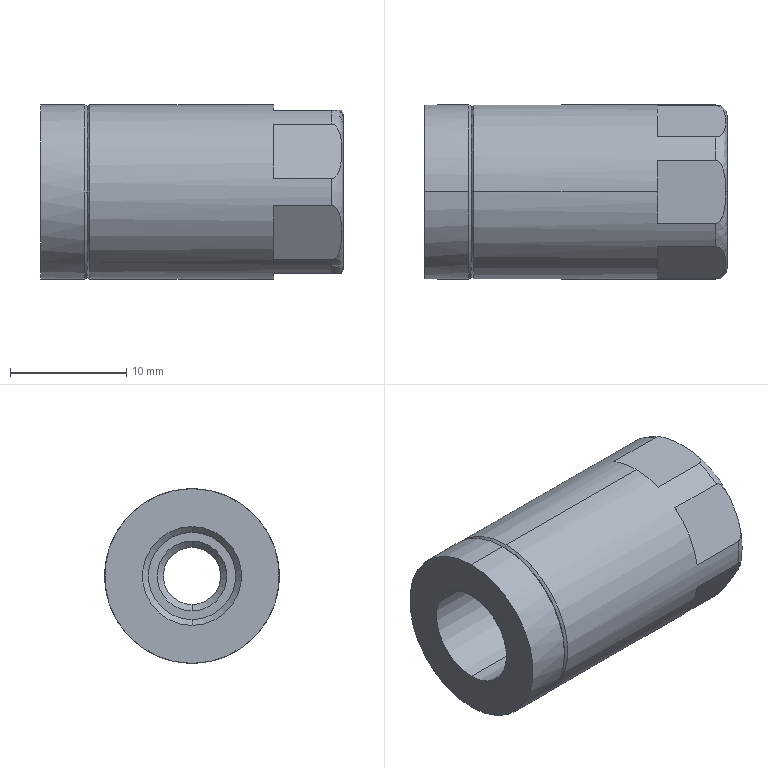Part | STEP file | _ACQJ-16x10_stoper | 1 solid | 35 faces | box 26 x 15 x 15 mm | volume 3348 mm3 | plane 15 | cone 10 | cylinder 8 | spline 2 | commonest cylinder face diameters 15 x4 4.917 x2 8.5 x2
STEP:
#1=CARTESIAN_POINT('',(26.,0.,-6.5));
#2=VERTEX_POINT('',#1);
#3=CARTESIAN_POINT('',(26.,0.,6.5));
#4=VERTEX_POINT('',#3);
#5=CARTESIAN_POINT('',(26.,0.,-6.5));
#6=CARTESIAN_POINT('',(26.,-13.,-6.5));
#7=CARTESIAN_POINT('',(26.,-13.,6.5));
#8=CARTESIAN_POINT('',(26.,0.,6.5));
#9=(BOUNDED_CURVE()B_SPLINE_CURVE(3,(#5,#6,#7,#8),.UNSPECIFIED.,.F.,.T.)B_SPLINE_CURVE_WITH_KNOTS((4,4),(0.,0.5),.UNSPECIFIED.)CURVE()GEOMETRIC_REPRESENTATION_ITEM()RATIONAL_B_SPLINE_CURVE((1.,0.3333,0.3333,1.))REPRESENTATION_ITEM(''));
#10=EDGE_CURVE('',#2,#4,#9,.T.);
#11=ORIENTED_EDGE('',*,*,#10,.T.);
#12=CARTESIAN_POINT('',(25.866,0.,7.));
#13=VERTEX_POINT('',#12);
#14=CARTESIAN_POINT('',(25.,0.,6.5));
#15=DIRECTION('',(0.,-1.,0.));
#16=DIRECTION('',(0.,0.,1.));
#17=AXIS2_PLACEMENT_3D('',#14,#15,#16);
#18=CIRCLE('',#17,1.);
#19=EDGE_CURVE('',#4,#13,#18,.T.);
#20=ORIENTED_EDGE('',*,*,#19,.T.);
#21=CARTESIAN_POINT('',(25.,-2.693,7.));
#22=VERTEX_POINT('',#21);
#23=CARTESIAN_POINT('',(25.866,0.,7.));
#24=CARTESIAN_POINT('',(25.866,-0.2506,7.));
#25=CARTESIAN_POINT('',(25.859,-0.5008,7.));
#26=CARTESIAN_POINT('',(25.825,-0.9999,7.));
#27=CARTESIAN_POINT('',(25.798,-1.249,7.));
#28=CARTESIAN_POINT('',(25.708,-1.744,7.));
#29=CARTESIAN_POINT('',(25.645,-1.991,7.));
#30=CARTESIAN_POINT('',(25.485,-2.33,7.));
#31=CARTESIAN_POINT('',(25.42,-2.44,7.));
#32=CARTESIAN_POINT('',(25.287,-2.576,7.));
#33=CARTESIAN_POINT('',(25.238,-2.616,7.));
#34=CARTESIAN_POINT('',(25.126,-2.675,7.));
#35=CARTESIAN_POINT('',(25.064,-2.693,7.));
#36=CARTESIAN_POINT('',(25.,-2.693,7.));
#37=B_SPLINE_CURVE_WITH_KNOTS('',3,(#23,#24,#25,#26,#27,#28,#29,#30,#31,#32,#33,#34,#35,#36),.UNSPECIFIED.,.F.,.F.,(4,2,2,2,2,2,4),(0.003036,0.003796,0.004556,0.005316,0.005696,0.005886,0.006076),.UNSPECIFIED.);
#38=EDGE_CURVE('',#13,#22,#37,.T.);
#39=ORIENTED_EDGE('',*,*,#38,.T.);
#40=CARTESIAN_POINT('',(25.,-4.716,5.832));
#41=VERTEX_POINT('',#40);
#42=CARTESIAN_POINT('',(25.,0.,0.));
#43=DIRECTION('',(-1.,0.,0.));
#44=DIRECTION('',(0.,0.,1.));
#45=AXIS2_PLACEMENT_3D('',#42,#43,#44);
#46=CIRCLE('',#45,7.5);
#47=EDGE_CURVE('',#41,#22,#46,.T.);
#48=ORIENTED_EDGE('',*,*,#47,.F.);
#49=CARTESIAN_POINT('',(25.,-7.408,1.168));
#50=VERTEX_POINT('',#49);
#51=CARTESIAN_POINT('',(25.,-4.716,5.832));
#52=CARTESIAN_POINT('',(25.064,-4.716,5.832));
#53=CARTESIAN_POINT('',(25.127,-4.725,5.816));
#54=CARTESIAN_POINT('',(25.239,-4.754,5.765));
#55=CARTESIAN_POINT('',(25.289,-4.775,5.73));
#56=CARTESIAN_POINT('',(25.421,-4.843,5.611));
#57=CARTESIAN_POINT('',(25.487,-4.899,5.515));
#58=CARTESIAN_POINT('',(25.594,-5.012,5.318));
#59=CARTESIAN_POINT('',(25.635,-5.072,5.214));
#60=CARTESIAN_POINT('',(25.704,-5.194,5.004));
#61=CARTESIAN_POINT('',(25.731,-5.255,4.898));
#62=CARTESIAN_POINT('',(25.798,-5.439,4.579));
#63=CARTESIAN_POINT('',(25.825,-5.563,4.364));
#64=CARTESIAN_POINT('',(25.859,-5.812,3.933));
#65=CARTESIAN_POINT('',(25.866,-5.938,3.715));
#66=CARTESIAN_POINT('',(25.866,-6.188,3.282));
#67=CARTESIAN_POINT('',(25.859,-6.313,3.065));
#68=CARTESIAN_POINT('',(25.824,-6.563,2.633));
#69=CARTESIAN_POINT('',(25.798,-6.687,2.417));
#70=CARTESIAN_POINT('',(25.707,-6.935,1.989));
#71=CARTESIAN_POINT('',(25.645,-7.058,1.776));
#72=CARTESIAN_POINT('',(25.485,-7.227,1.482));
#73=CARTESIAN_POINT('',(25.419,-7.282,1.387));
#74=CARTESIAN_POINT('',(25.287,-7.35,1.269));
#75=CARTESIAN_POINT('',(25.238,-7.37,1.234));
#76=CARTESIAN_POINT('',(25.126,-7.4,1.183));
#77=CARTESIAN_POINT('',(25.064,-7.408,1.168));
#78=CARTESIAN_POINT('',(25.,-7.408,1.168));
#79=B_SPLINE_CURVE_WITH_KNOTS('',3,(#51,#52,#53,#54,#55,#56,#57,#58,#59,#60,#61,#62,#63,#64,#65,#66,#67,#68,#69,#70,#71,#72,#73,#74,#75,#76,#77,#78),.UNSPECIFIED.,.F.,.F.,(4,2,2,2,2,2,2,2,2,2,2,2,2,4),(0.,0.0001899,0.0003798,0.0007595,0.001139,0.001519,0.002279,0.003038,0.003798,0.004557,0.005317,0.005697,0.005887,0.006076),.UNSPECIFIED.);
#80=EDGE_CURVE('',#41,#50,#79,.T.);
#81=ORIENTED_EDGE('',*,*,#80,.T.);
#82=CARTESIAN_POINT('',(25.,-7.408,-1.168));
#83=VERTEX_POINT('',#82);
#84=CARTESIAN_POINT('',(25.,0.,0.));
#85=DIRECTION('',(-1.,0.,0.));
#86=DIRECTION('',(0.,0.,1.));
#87=AXIS2_PLACEMENT_3D('',#84,#85,#86);
#88=CIRCLE('',#87,7.5);
#89=EDGE_CURVE('',#83,#50,#88,.T.);
#90=ORIENTED_EDGE('',*,*,#89,.F.);
#91=CARTESIAN_POINT('',(25.,-4.716,-5.832));
#92=VERTEX_POINT('',#91);
#93=CARTESIAN_POINT('',(25.,-7.408,-1.168));
#94=CARTESIAN_POINT('',(25.064,-7.408,-1.168));
#95=CARTESIAN_POINT('',(25.127,-7.4,-1.184));
#96=CARTESIAN_POINT('',(25.239,-7.37,-1.235));
#97=CARTESIAN_POINT('',(25.289,-7.35,-1.27));
#98=CARTESIAN_POINT('',(25.421,-7.281,-1.389));
#99=CARTESIAN_POINT('',(25.487,-7.226,-1.485));
#100=CARTESIAN_POINT('',(25.594,-7.112,-1.682));
#101=CARTESIAN_POINT('',(25.635,-7.052,-1.786));
#102=CARTESIAN_POINT('',(25.704,-6.931,-1.996));
#103=CARTESIAN_POINT('',(25.731,-6.87,-2.102));
#104=CARTESIAN_POINT('',(25.798,-6.685,-2.421));
#105=CARTESIAN_POINT('',(25.825,-6.561,-2.636));
#106=CARTESIAN_POINT('',(25.859,-6.312,-3.067));
#107=CARTESIAN_POINT('',(25.866,-6.187,-3.285));
#108=CARTESIAN_POINT('',(25.866,-5.936,-3.718));
#109=CARTESIAN_POINT('',(25.859,-5.811,-3.935));
#110=CARTESIAN_POINT('',(25.824,-5.562,-4.367));
#111=CARTESIAN_POINT('',(25.798,-5.437,-4.583));
#112=CARTESIAN_POINT('',(25.707,-5.19,-5.011));
#113=CARTESIAN_POINT('',(25.645,-5.067,-5.224));
#114=CARTESIAN_POINT('',(25.485,-4.897,-5.518));
#115=CARTESIAN_POINT('',(25.419,-4.842,-5.613));
#116=CARTESIAN_POINT('',(25.287,-4.774,-5.731));
#117=CARTESIAN_POINT('',(25.238,-4.754,-5.766));
#118=CARTESIAN_POINT('',(25.126,-4.725,-5.817));
#119=CARTESIAN_POINT('',(25.064,-4.716,-5.832));
#120=CARTESIAN_POINT('',(25.,-4.716,-5.832));
#121=B_SPLINE_CURVE_WITH_KNOTS('',3,(#93,#94,#95,#96,#97,#98,#99,#100,#101,#102,#103,#104,#105,#106,#107,#108,#109,#110,#111,#112,#113,#114,#115,#116,#117,#118,#119,#120),.UNSPECIFIED.,.F.,.F.,(4,2,2,2,2,2,2,2,2,2,2,2,2,4),(0.,0.0001899,0.0003798,0.0007595,0.001139,0.001519,0.002279,0.003038,0.003798,0.004557,0.005317,0.005697,0.005887,0.006076),.UNSPECIFIED.);
#122=EDGE_CURVE('',#83,#92,#121,.T.);
#123=ORIENTED_EDGE('',*,*,#122,.T.);
#124=CARTESIAN_POINT('',(25.,-2.693,-7.));
#125=VERTEX_POINT('',#124);
#126=CARTESIAN_POINT('',(25.,0.,0.));
#127=DIRECTION('',(-1.,0.,0.));
#128=DIRECTION('',(0.,0.,1.));
#129=AXIS2_PLACEMENT_3D('',#126,#127,#128);
#130=CIRCLE('',#129,7.5);
#131=EDGE_CURVE('',#125,#92,#130,.T.);
#132=ORIENTED_EDGE('',*,*,#131,.F.);
#133=CARTESIAN_POINT('',(25.866,0.,-7.));
#134=VERTEX_POINT('',#133);
#135=CARTESIAN_POINT('',(25.,-2.693,-7.));
#136=CARTESIAN_POINT('',(25.064,-2.693,-7.));
#137=CARTESIAN_POINT('',(25.127,-2.675,-7.));
#138=CARTESIAN_POINT('',(25.239,-2.616,-7.));
#139=CARTESIAN_POINT('',(25.289,-2.575,-7.));
#140=CARTESIAN_POINT('',(25.421,-2.438,-7.));
#141=CARTESIAN_POINT('',(25.486,-2.327,-7.));
#142=CARTESIAN_POINT('',(25.593,-2.1,-7.));
#143=CARTESIAN_POINT('',(25.635,-1.98,-7.));
#144=CARTESIAN_POINT('',(25.704,-1.738,-7.));
#145=CARTESIAN_POINT('',(25.731,-1.616,-7.));
#146=CARTESIAN_POINT('',(25.798,-1.247,-7.));
#147=CARTESIAN_POINT('',(25.825,-0.9993,-7.));
#148=CARTESIAN_POINT('',(25.859,-0.5011,-7.));
#149=CARTESIAN_POINT('',(25.866,-0.2503,-7.));
#150=CARTESIAN_POINT('',(25.866,0.,-7.));
#151=B_SPLINE_CURVE_WITH_KNOTS('',3,(#135,#136,#137,#138,#139,#140,#141,#142,#143,#144,#145,#146,#147,#148,#149,#150),.UNSPECIFIED.,.F.,.F.,(4,2,2,2,2,2,2,4),(0.,0.0001898,0.0003795,0.0007591,0.001139,0.001518,0.002277,0.003036),.UNSPECIFIED.);
#152=EDGE_CURVE('',#125,#134,#151,.T.);
#153=ORIENTED_EDGE('',*,*,#152,.T.);
#154=CARTESIAN_POINT('',(25.,0.,-6.5));
#155=DIRECTION('',(0.,1.,0.));
#156=DIRECTION('',(0.,0.,-1.));
#157=AXIS2_PLACEMENT_3D('',#154,#155,#156);
#158=CIRCLE('',#157,1.);
#159=EDGE_CURVE('',#2,#134,#158,.T.);
#160=ORIENTED_EDGE('',*,*,#159,.F.);
#161=EDGE_LOOP('',(#11,#20,#39,#48,#81,#90,#123,#132,#153,#160));
#162=FACE_OUTER_BOUND('',#161,.T.);
#163=CARTESIAN_POINT('',(26.,0.,6.5));
#164=CARTESIAN_POINT('',(26.,-13.,6.5));
#165=CARTESIAN_POINT('',(26.,-13.,-6.5));
#166=CARTESIAN_POINT('',(26.,0.,-6.5));
#167=CARTESIAN_POINT('',(26.,0.,7.086));
#168=CARTESIAN_POINT('',(26.,-14.172,7.086));
#169=CARTESIAN_POINT('',(26.,-14.172,-7.086));
#170=CARTESIAN_POINT('',(26.,0.,-7.086));
#171=CARTESIAN_POINT('',(25.586,0.,7.5));
#172=CARTESIAN_POINT('',(25.586,-15.,7.5));
#173=CARTESIAN_POINT('',(25.586,-15.,-7.5));
#174=CARTESIAN_POINT('',(25.586,0.,-7.5));
#175=CARTESIAN_POINT('',(25.,0.,7.5));
#176=CARTESIAN_POINT('',(25.,-15.,7.5));
#177=CARTESIAN_POINT('',(25.,-15.,-7.5));
#178=CARTESIAN_POINT('',(25.,0.,-7.5));
#179=(BOUNDED_SURFACE()B_SPLINE_SURFACE(3,3,((#163,#164,#165,#166),(#167,#168,#169,#170),(#171,#172,#173,#174),(#175,#176,#177,#178)),.UNSPECIFIED.,.F.,.F.,.F.)B_SPLINE_SURFACE_WITH_KNOTS((4,4),(4,4),(0.,1.),(0.,1.),.UNSPECIFIED.)GEOMETRIC_REPRESENTATION_ITEM()RATIONAL_B_SPLINE_SURFACE(((1.,0.3333,0.3333,1.),(0.8047,0.2682,0.2682,0.8047),(0.8047,0.2682,0.2682,0.8047),(1.,0.3333,0.3333,1.)))REPRESENTATION_ITEM('')SURFACE());
#180=ADVANCED_FACE('',(#162),#179,.T.);
#181=CARTESIAN_POINT('',(20.,2.693,-7.));
#182=VERTEX_POINT('',#181);
#183=CARTESIAN_POINT('',(20.,0.,-7.5));
#184=VERTEX_POINT('',#183);
#185=CARTESIAN_POINT('',(20.,0.,0.));
#186=DIRECTION('',(-1.,0.,0.));
#187=DIRECTION('',(0.,0.,1.));
#188=AXIS2_PLACEMENT_3D('',#185,#186,#187);
#189=CIRCLE('',#188,7.5);
#190=EDGE_CURVE('',#182,#184,#189,.T.);
#191=ORIENTED_EDGE('',*,*,#190,.T.);
#192=CARTESIAN_POINT('',(4.2,0.,-7.5));
#193=VERTEX_POINT('',#192);
#194=CARTESIAN_POINT('',(26.,0.,-7.5));
#195=DIRECTION('',(-1.,0.,0.));
#196=VECTOR('',#195,1000.);
#197=LINE('',#194,#196);
#198=EDGE_CURVE('',#184,#193,#197,.T.);
#199=ORIENTED_EDGE('',*,*,#198,.T.);
#200=CARTESIAN_POINT('',(4.2,0.,7.5));
#201=VERTEX_POINT('',#200);
#202=CARTESIAN_POINT('',(4.2,0.,0.));
#203=DIRECTION('',(1.,0.,0.));
#204=DIRECTION('',(0.,0.,1.));
#205=AXIS2_PLACEMENT_3D('',#202,#203,#204);
#206=CIRCLE('',#205,7.5);
#207=EDGE_CURVE('',#193,#201,#206,.T.);
#208=ORIENTED_EDGE('',*,*,#207,.T.);
#209=CARTESIAN_POINT('',(20.,0.,7.5));
#210=VERTEX_POINT('',#209);
#211=CARTESIAN_POINT('',(26.,0.,7.5));
#212=DIRECTION('',(-1.,0.,0.));
#213=VECTOR('',#212,1000.);
#214=LINE('',#211,#213);
#215=EDGE_CURVE('',#210,#201,#214,.T.);
#216=ORIENTED_EDGE('',*,*,#215,.F.);
#217=CARTESIAN_POINT('',(20.,2.693,7.));
#218=VERTEX_POINT('',#217);
#219=CARTESIAN_POINT('',(20.,0.,0.));
#220=DIRECTION('',(-1.,0.,0.));
#221=DIRECTION('',(0.,0.,1.));
#222=AXIS2_PLACEMENT_3D('',#219,#220,#221);
#223=CIRCLE('',#222,7.5);
#224=EDGE_CURVE('',#210,#218,#223,.T.);
#225=ORIENTED_EDGE('',*,*,#224,.T.);
#226=CARTESIAN_POINT('',(25.,2.693,7.));
#227=VERTEX_POINT('',#226);
#228=CARTESIAN_POINT('',(26.,2.693,7.));
#229=DIRECTION('',(1.,0.,0.));
#230=VECTOR('',#229,1000.);
#231=LINE('',#228,#230);
#232=EDGE_CURVE('',#218,#227,#231,.T.);
#233=ORIENTED_EDGE('',*,*,#232,.T.);
#234=CARTESIAN_POINT('',(25.,4.716,5.832));
#235=VERTEX_POINT('',#234);
#236=CARTESIAN_POINT('',(25.,0.,0.));
#237=DIRECTION('',(-1.,0.,0.));
#238=DIRECTION('',(0.,0.,1.));
#239=AXIS2_PLACEMENT_3D('',#236,#237,#238);
#240=CIRCLE('',#239,7.5);
#241=EDGE_CURVE('',#227,#235,#240,.T.);
#242=ORIENTED_EDGE('',*,*,#241,.T.);
#243=CARTESIAN_POINT('',(20.,4.716,5.832));
#244=VERTEX_POINT('',#243);
#245=CARTESIAN_POINT('',(26.,4.716,5.832));
#246=DIRECTION('',(-1.,0.,0.));
#247=VECTOR('',#246,1000.);
#248=LINE('',#245,#247);
#249=EDGE_CURVE('',#235,#244,#248,.T.);
#250=ORIENTED_EDGE('',*,*,#249,.T.);
#251=CARTESIAN_POINT('',(20.,7.408,1.168));
#252=VERTEX_POINT('',#251);
#253=CARTESIAN_POINT('',(20.,0.,0.));
#254=DIRECTION('',(-1.,0.,0.));
#255=DIRECTION('',(0.,0.,1.));
#256=AXIS2_PLACEMENT_3D('',#253,#254,#255);
#257=CIRCLE('',#256,7.5);
#258=EDGE_CURVE('',#244,#252,#257,.T.);
#259=ORIENTED_EDGE('',*,*,#258,.T.);
#260=CARTESIAN_POINT('',(25.,7.408,1.168));
#261=VERTEX_POINT('',#260);
#262=CARTESIAN_POINT('',(26.,7.408,1.168));
#263=DIRECTION('',(1.,0.,0.));
#264=VECTOR('',#263,1000.);
#265=LINE('',#262,#264);
#266=EDGE_CURVE('',#252,#261,#265,.T.);
#267=ORIENTED_EDGE('',*,*,#266,.T.);
#268=CARTESIAN_POINT('',(25.,7.408,-1.168));
#269=VERTEX_POINT('',#268);
#270=CARTESIAN_POINT('',(25.,0.,0.));
#271=DIRECTION('',(-1.,0.,0.));
#272=DIRECTION('',(0.,0.,1.));
#273=AXIS2_PLACEMENT_3D('',#270,#271,#272);
#274=CIRCLE('',#273,7.5);
#275=EDGE_CURVE('',#261,#269,#274,.T.);
#276=ORIENTED_EDGE('',*,*,#275,.T.);
#277=CARTESIAN_POINT('',(20.,7.408,-1.168));
#278=VERTEX_POINT('',#277);
#279=CARTESIAN_POINT('',(26.,7.408,-1.168));
#280=DIRECTION('',(-1.,0.,0.));
#281=VECTOR('',#280,1000.);
#282=LINE('',#279,#281);
#283=EDGE_CURVE('',#269,#278,#282,.T.);
#284=ORIENTED_EDGE('',*,*,#283,.T.);
#285=CARTESIAN_POINT('',(20.,4.716,-5.832));
#286=VERTEX_POINT('',#285);
#287=CARTESIAN_POINT('',(20.,0.,0.));
#288=DIRECTION('',(-1.,0.,0.));
#289=DIRECTION('',(0.,0.,1.));
#290=AXIS2_PLACEMENT_3D('',#287,#288,#289);
#291=CIRCLE('',#290,7.5);
#292=EDGE_CURVE('',#278,#286,#291,.T.);
#293=ORIENTED_EDGE('',*,*,#292,.T.);
#294=CARTESIAN_POINT('',(25.,4.716,-5.832));
#295=VERTEX_POINT('',#294);
#296=CARTESIAN_POINT('',(26.,4.716,-5.832));
#297=DIRECTION('',(1.,0.,0.));
#298=VECTOR('',#297,1000.);
#299=LINE('',#296,#298);
#300=EDGE_CURVE('',#286,#295,#299,.T.);
#301=ORIENTED_EDGE('',*,*,#300,.T.);
#302=CARTESIAN_POINT('',(25.,2.693,-7.));
#303=VERTEX_POINT('',#302);
#304=CARTESIAN_POINT('',(25.,0.,0.));
#305=DIRECTION('',(-1.,0.,0.));
#306=DIRECTION('',(0.,0.,1.));
#307=AXIS2_PLACEMENT_3D('',#304,#305,#306);
#308=CIRCLE('',#307,7.5);
#309=EDGE_CURVE('',#295,#303,#308,.T.);
#310=ORIENTED_EDGE('',*,*,#309,.T.);
#311=CARTESIAN_POINT('',(26.,2.693,-7.));
#312=DIRECTION('',(-1.,0.,0.));
#313=VECTOR('',#312,1000.);
#314=LINE('',#311,#313);
#315=EDGE_CURVE('',#303,#182,#314,.T.);
#316=ORIENTED_EDGE('',*,*,#315,.T.);
#317=EDGE_LOOP('',(#191,#199,#208,#216,#225,#233,#242,#250,#259,#267,#276,#284,#293,#301,#310,#316));
#318=FACE_OUTER_BOUND('',#317,.T.);
#319=CARTESIAN_POINT('',(26.,0.,0.));
#320=DIRECTION('',(-1.,0.,0.));
#321=DIRECTION('',(0.,0.,1.));
#322=AXIS2_PLACEMENT_3D('',#319,#320,#321);
#323=CYLINDRICAL_SURFACE('',#322,7.5);
#324=ADVANCED_FACE('',(#318),#323,.T.);
#325=CARTESIAN_POINT('',(4.,7.3,0.));
#326=VERTEX_POINT('',#325);
#327=CARTESIAN_POINT('',(4.,0.,7.3));
#328=VERTEX_POINT('',#327);
#329=CARTESIAN_POINT('',(4.,0.,0.));
#330=DIRECTION('',(1.,0.,0.));
#331=DIRECTION('',(0.,0.,-1.));
#332=AXIS2_PLACEMENT_3D('',#329,#330,#331);
#333=CIRCLE('',#332,7.3);
#334=EDGE_CURVE('',#326,#328,#333,.T.);
#335=ORIENTED_EDGE('',*,*,#334,.T.);
#336=CARTESIAN_POINT('',(4.2,0.,7.5));
#337=DIRECTION('',(0.7071,0.,0.7071));
#338=VECTOR('',#337,1000.);
#339=LINE('',#336,#338);
#340=EDGE_CURVE('',#328,#201,#339,.T.);
#341=ORIENTED_EDGE('',*,*,#340,.T.);
#342=ORIENTED_EDGE('',*,*,#207,.F.);
#343=CARTESIAN_POINT('',(4.,0.,-7.3));
#344=VERTEX_POINT('',#343);
#345=CARTESIAN_POINT('',(4.2,0.,-7.5));
#346=DIRECTION('',(0.7071,0.,-0.7071));
#347=VECTOR('',#346,1000.);
#348=LINE('',#345,#347);
#349=EDGE_CURVE('',#344,#193,#348,.T.);
#350=ORIENTED_EDGE('',*,*,#349,.F.);
#351=CARTESIAN_POINT('',(4.,0.,0.));
#352=DIRECTION('',(1.,0.,0.));
#353=DIRECTION('',(0.,0.,-1.));
#354=AXIS2_PLACEMENT_3D('',#351,#352,#353);
#355=CIRCLE('',#354,7.3);
#356=EDGE_CURVE('',#344,#326,#355,.T.);
#357=ORIENTED_EDGE('',*,*,#356,.T.);
#358=EDGE_LOOP('',(#335,#341,#342,#350,#357));
#359=FACE_OUTER_BOUND('',#358,.T.);
#360=CARTESIAN_POINT('',(4.2,0.,0.));
#361=DIRECTION('',(1.,0.,0.));
#362=DIRECTION('',(0.,0.,-1.));
#363=AXIS2_PLACEMENT_3D('',#360,#361,#362);
#364=CONICAL_SURFACE('',#363,7.5,0.7854);
#365=ADVANCED_FACE('',(#359),#364,.T.);
#366=ORIENTED_EDGE('',*,*,#334,.F.);
#367=CARTESIAN_POINT('',(3.8,7.5,0.));
#368=VERTEX_POINT('',#367);
#369=CARTESIAN_POINT('',(3.8,7.5,0.));
#370=DIRECTION('',(-0.7071,0.7071,0.));
#371=VECTOR('',#370,1000.);
#372=LINE('',#369,#371);
#373=EDGE_CURVE('',#326,#368,#372,.T.);
#374=ORIENTED_EDGE('',*,*,#373,.T.);
#375=CARTESIAN_POINT('',(3.8,0.,7.5));
#376=VERTEX_POINT('',#375);
#377=CARTESIAN_POINT('',(3.8,0.,0.));
#378=DIRECTION('',(1.,0.,0.));
#379=DIRECTION('',(0.,0.,1.));
#380=AXIS2_PLACEMENT_3D('',#377,#378,#379);
#381=CIRCLE('',#380,7.5);
#382=EDGE_CURVE('',#368,#376,#381,.T.);
#383=ORIENTED_EDGE('',*,*,#382,.T.);
#384=CARTESIAN_POINT('',(3.8,-7.5,0.));
#385=VERTEX_POINT('',#384);
#386=CARTESIAN_POINT('',(3.8,0.,0.));
#387=DIRECTION('',(1.,0.,0.));
#388=DIRECTION('',(0.,0.,1.));
#389=AXIS2_PLACEMENT_3D('',#386,#387,#388);
#390=CIRCLE('',#389,7.5);
#391=EDGE_CURVE('',#376,#385,#390,.T.);
#392=ORIENTED_EDGE('',*,*,#391,.T.);
#393=CARTESIAN_POINT('',(4.,-7.3,0.));
#394=VERTEX_POINT('',#393);
#395=CARTESIAN_POINT('',(3.8,-7.5,0.));
#396=DIRECTION('',(-0.7071,-0.7071,0.));
#397=VECTOR('',#396,1000.);
#398=LINE('',#395,#397);
#399=EDGE_CURVE('',#394,#385,#398,.T.);
#400=ORIENTED_EDGE('',*,*,#399,.F.);
#401=CARTESIAN_POINT('',(4.,0.,0.));
#402=DIRECTION('',(1.,0.,0.));
#403=DIRECTION('',(0.,0.,-1.));
#404=AXIS2_PLACEMENT_3D('',#401,#402,#403);
#405=CIRCLE('',#404,7.3);
#406=EDGE_CURVE('',#328,#394,#405,.T.);
#407=ORIENTED_EDGE('',*,*,#406,.F.);
#408=EDGE_LOOP('',(#366,#374,#383,#392,#400,#407));
#409=FACE_OUTER_BOUND('',#408,.T.);
#410=CARTESIAN_POINT('',(3.8,0.,0.));
#411=DIRECTION('',(-1.,0.,0.));
#412=DIRECTION('',(0.,-1.,0.));
#413=AXIS2_PLACEMENT_3D('',#410,#411,#412);
#414=CONICAL_SURFACE('',#413,7.5,0.7854);
#415=ADVANCED_FACE('',(#409),#414,.T.);
#416=CARTESIAN_POINT('',(3.8,0.,-7.5));
#417=VERTEX_POINT('',#416);
#418=CARTESIAN_POINT('',(3.8,0.,0.));
#419=DIRECTION('',(1.,0.,0.));
#420=DIRECTION('',(0.,0.,1.));
#421=AXIS2_PLACEMENT_3D('',#418,#419,#420);
#422=CIRCLE('',#421,7.5);
#423=EDGE_CURVE('',#417,#368,#422,.T.);
#424=ORIENTED_EDGE('',*,*,#423,.F.);
#425=CARTESIAN_POINT('',(0.,0.,-7.5));
#426=VERTEX_POINT('',#425);
#427=CARTESIAN_POINT('',(26.,0.,-7.5));
#428=DIRECTION('',(-1.,0.,0.));
#429=VECTOR('',#428,1000.);
#430=LINE('',#427,#429);
#431=EDGE_CURVE('',#417,#426,#430,.T.);
#432=ORIENTED_EDGE('',*,*,#431,.T.);
#433=CARTESIAN_POINT('',(0.,0.,7.5));
#434=VERTEX_POINT('',#433);
#435=CARTESIAN_POINT('',(0.,0.,0.));
#436=DIRECTION('',(1.,0.,0.));
#437=DIRECTION('',(0.,0.,1.));
#438=AXIS2_PLACEMENT_3D('',#435,#436,#437);
#439=CIRCLE('',#438,7.5);
#440=EDGE_CURVE('',#426,#434,#439,.T.);
#441=ORIENTED_EDGE('',*,*,#440,.T.);
#442=CARTESIAN_POINT('',(26.,0.,7.5));
#443=DIRECTION('',(-1.,0.,0.));
#444=VECTOR('',#443,1000.);
#445=LINE('',#442,#444);
#446=EDGE_CURVE('',#376,#434,#445,.T.);
#447=ORIENTED_EDGE('',*,*,#446,.F.);
#448=ORIENTED_EDGE('',*,*,#382,.F.);
#449=EDGE_LOOP('',(#424,#432,#441,#447,#448));
#450=FACE_OUTER_BOUND('',#449,.T.);
#451=CARTESIAN_POINT('',(26.,0.,0.));
#452=DIRECTION('',(-1.,0.,0.));
#453=DIRECTION('',(0.,0.,1.));
#454=AXIS2_PLACEMENT_3D('',#451,#452,#453);
#455=CYLINDRICAL_SURFACE('',#454,7.5);
#456=ADVANCED_FACE('',(#450),#455,.T.);
#457=CARTESIAN_POINT('',(25.459,0.,2.458));
#458=VERTEX_POINT('',#457);
#459=CARTESIAN_POINT('',(25.459,0.,-2.458));
#460=VERTEX_POINT('',#459);
#461=CARTESIAN_POINT('',(25.459,0.,0.));
#462=DIRECTION('',(1.,0.,0.));
#463=DIRECTION('',(0.,0.,-1.));
#464=AXIS2_PLACEMENT_3D('',#461,#462,#463);
#465=CIRCLE('',#464,2.458);
#466=EDGE_CURVE('',#458,#460,#465,.T.);
#467=ORIENTED_EDGE('',*,*,#466,.F.);
#468=CARTESIAN_POINT('',(26.,0.,3.));
#469=VERTEX_POINT('',#468);
#470=CARTESIAN_POINT('',(26.,0.,3.));
#471=DIRECTION('',(0.7071,0.,0.7071));
#472=VECTOR('',#471,1000.);
#473=LINE('',#470,#472);
#474=EDGE_CURVE('',#458,#469,#473,.T.);
#475=ORIENTED_EDGE('',*,*,#474,.T.);
#476=CARTESIAN_POINT('',(26.,0.,-3.));
#477=VERTEX_POINT('',#476);
#478=CARTESIAN_POINT('',(26.,0.,0.));
#479=DIRECTION('',(1.,0.,0.));
#480=DIRECTION('',(0.,0.,-1.));
#481=AXIS2_PLACEMENT_3D('',#478,#479,#480);
#482=CIRCLE('',#481,3.);
#483=EDGE_CURVE('',#469,#477,#482,.T.);
#484=ORIENTED_EDGE('',*,*,#483,.T.);
#485=CARTESIAN_POINT('',(26.,0.,-3.));
#486=DIRECTION('',(0.7071,0.,-0.7071));
#487=VECTOR('',#486,1000.);
#488=LINE('',#485,#487);
#489=EDGE_CURVE('',#460,#477,#488,.T.);
#490=ORIENTED_EDGE('',*,*,#489,.F.);
#491=EDGE_LOOP('',(#467,#475,#484,#490));
#492=FACE_OUTER_BOUND('',#491,.T.);
#493=CARTESIAN_POINT('',(26.,0.,0.));
#494=DIRECTION('',(1.,0.,0.));
#495=DIRECTION('',(0.,0.,-1.));
#496=AXIS2_PLACEMENT_3D('',#493,#494,#495);
#497=CONICAL_SURFACE('',#496,3.,0.7854);
#498=ADVANCED_FACE('',(#492),#497,.F.);
#499=ORIENTED_EDGE('',*,*,#466,.T.);
#500=CARTESIAN_POINT('',(18.541,0.,-2.458));
#501=VERTEX_POINT('',#500);
#502=CARTESIAN_POINT('',(26.,0.,-2.458));
#503=DIRECTION('',(-1.,0.,0.));
#504=VECTOR('',#503,1000.);
#505=LINE('',#502,#504);
#506=EDGE_CURVE('',#460,#501,#505,.T.);
#507=ORIENTED_EDGE('',*,*,#506,.T.);
#508=CARTESIAN_POINT('',(18.541,0.,2.458));
#509=VERTEX_POINT('',#508);
#510=CARTESIAN_POINT('',(18.541,0.,0.));
#511=DIRECTION('',(1.,0.,0.));
#512=DIRECTION('',(0.,0.,1.));
#513=AXIS2_PLACEMENT_3D('',#510,#511,#512);
#514=CIRCLE('',#513,2.458);
#515=EDGE_CURVE('',#509,#501,#514,.T.);
#516=ORIENTED_EDGE('',*,*,#515,.F.);
#517=CARTESIAN_POINT('',(26.,0.,2.458));
#518=DIRECTION('',(-1.,0.,0.));
#519=VECTOR('',#518,1000.);
#520=LINE('',#517,#519);
#521=EDGE_CURVE('',#458,#509,#520,.T.);
#522=ORIENTED_EDGE('',*,*,#521,.F.);
#523=EDGE_LOOP('',(#499,#507,#516,#522));
#524=FACE_OUTER_BOUND('',#523,.T.);
#525=CARTESIAN_POINT('',(26.,0.,0.));
#526=DIRECTION('',(-1.,0.,0.));
#527=DIRECTION('',(0.,0.,1.));
#528=AXIS2_PLACEMENT_3D('',#525,#526,#527);
#529=CYLINDRICAL_SURFACE('',#528,2.458);
#530=ADVANCED_FACE('',(#524),#529,.F.);
#531=CARTESIAN_POINT('',(17.5,0.,-4.25));
#532=VERTEX_POINT('',#531);
#533=CARTESIAN_POINT('',(17.5,0.,4.25));
#534=VERTEX_POINT('',#533);
#535=CARTESIAN_POINT('',(17.5,0.,0.));
#536=DIRECTION('',(-1.,0.,0.));
#537=DIRECTION('',(0.,0.,1.));
#538=AXIS2_PLACEMENT_3D('',#535,#536,#537);
#539=CIRCLE('',#538,4.25);
#540=EDGE_CURVE('',#532,#534,#539,.T.);
#541=ORIENTED_EDGE('',*,*,#540,.F.);
#542=CARTESIAN_POINT('',(0.,0.,-4.25));
#543=VERTEX_POINT('',#542);
#544=CARTESIAN_POINT('',(26.,0.,-4.25));
#545=DIRECTION('',(-1.,0.,0.));
#546=VECTOR('',#545,1000.);
#547=LINE('',#544,#546);
#548=EDGE_CURVE('',#532,#543,#547,.T.);
#549=ORIENTED_EDGE('',*,*,#548,.T.);
#550=CARTESIAN_POINT('',(0.,0.,4.25));
#551=VERTEX_POINT('',#550);
#552=CARTESIAN_POINT('',(0.,0.,0.));
#553=DIRECTION('',(-1.,0.,0.));
#554=DIRECTION('',(0.,0.,1.));
#555=AXIS2_PLACEMENT_3D('',#552,#553,#554);
#556=CIRCLE('',#555,4.25);
#557=EDGE_CURVE('',#543,#551,#556,.T.);
#558=ORIENTED_EDGE('',*,*,#557,.T.);
#559=CARTESIAN_POINT('',(26.,0.,4.25));
#560=DIRECTION('',(-1.,0.,0.));
#561=VECTOR('',#560,1000.);
#562=LINE('',#559,#561);
#563=EDGE_CURVE('',#534,#551,#562,.T.);
#564=ORIENTED_EDGE('',*,*,#563,.F.);
#565=EDGE_LOOP('',(#541,#549,#558,#564));
#566=FACE_OUTER_BOUND('',#565,.T.);
#567=CARTESIAN_POINT('',(26.,0.,0.));
#568=DIRECTION('',(-1.,0.,0.));
#569=DIRECTION('',(0.,0.,1.));
#570=AXIS2_PLACEMENT_3D('',#567,#568,#569);
#571=CYLINDRICAL_SURFACE('',#570,4.25);
#572=ADVANCED_FACE('',(#566),#571,.F.);
#573=ORIENTED_EDGE('',*,*,#515,.T.);
#574=CARTESIAN_POINT('',(18.,0.,-3.));
#575=VERTEX_POINT('',#574);
#576=CARTESIAN_POINT('',(18.,0.,-3.));
#577=DIRECTION('',(-0.7071,0.,-0.7071));
#578=VECTOR('',#577,1000.);
#579=LINE('',#576,#578);
#580=EDGE_CURVE('',#501,#575,#579,.T.);
#581=ORIENTED_EDGE('',*,*,#580,.T.);
#582=CARTESIAN_POINT('',(18.,0.,3.));
#583=VERTEX_POINT('',#582);
#584=CARTESIAN_POINT('',(18.,0.,0.));
#585=DIRECTION('',(1.,0.,0.));
#586=DIRECTION('',(0.,0.,1.));
#587=AXIS2_PLACEMENT_3D('',#584,#585,#586);
#588=CIRCLE('',#587,3.);
#589=EDGE_CURVE('',#583,#575,#588,.T.);
#590=ORIENTED_EDGE('',*,*,#589,.F.);
#591=CARTESIAN_POINT('',(18.,0.,3.));
#592=DIRECTION('',(-0.7071,0.,0.7071));
#593=VECTOR('',#592,1000.);
#594=LINE('',#591,#593);
#595=EDGE_CURVE('',#509,#583,#594,.T.);
#596=ORIENTED_EDGE('',*,*,#595,.F.);
#597=EDGE_LOOP('',(#573,#581,#590,#596));
#598=FACE_OUTER_BOUND('',#597,.T.);
#599=CARTESIAN_POINT('',(18.,0.,0.));
#600=DIRECTION('',(-1.,0.,0.));
#601=DIRECTION('',(0.,0.,1.));
#602=AXIS2_PLACEMENT_3D('',#599,#600,#601);
#603=CONICAL_SURFACE('',#602,3.,0.7854);
#604=ADVANCED_FACE('',(#598),#603,.F.);
#605=CARTESIAN_POINT('',(18.,0.,-3.75));
#606=VERTEX_POINT('',#605);
#607=CARTESIAN_POINT('',(18.,0.,3.75));
#608=VERTEX_POINT('',#607);
#609=CARTESIAN_POINT('',(18.,0.,0.));
#610=DIRECTION('',(-1.,0.,0.));
#611=DIRECTION('',(0.,0.,1.));
#612=AXIS2_PLACEMENT_3D('',#609,#610,#611);
#613=CIRCLE('',#612,3.75);
#614=EDGE_CURVE('',#606,#608,#613,.T.);
#615=ORIENTED_EDGE('',*,*,#614,.F.);
#616=CARTESIAN_POINT('',(17.5,0.,-4.25));
#617=DIRECTION('',(-0.7071,0.,-0.7071));
#618=VECTOR('',#617,1000.);
#619=LINE('',#616,#618);
#620=EDGE_CURVE('',#606,#532,#619,.T.);
#621=ORIENTED_EDGE('',*,*,#620,.T.);
#622=ORIENTED_EDGE('',*,*,#540,.T.);
#623=CARTESIAN_POINT('',(17.5,0.,4.25));
#624=DIRECTION('',(-0.7071,0.,0.7071));
#625=VECTOR('',#624,1000.);
#626=LINE('',#623,#625);
#627=EDGE_CURVE('',#608,#534,#626,.T.);
#628=ORIENTED_EDGE('',*,*,#627,.F.);
#629=EDGE_LOOP('',(#615,#621,#622,#628));
#630=FACE_OUTER_BOUND('',#629,.T.);
#631=CARTESIAN_POINT('',(17.5,0.,0.));
#632=DIRECTION('',(-1.,0.,0.));
#633=DIRECTION('',(0.,0.,1.));
#634=AXIS2_PLACEMENT_3D('',#631,#632,#633);
#635=CONICAL_SURFACE('',#634,4.25,0.7854);
#636=ADVANCED_FACE('',(#630),#635,.F.);
#637=ORIENTED_EDGE('',*,*,#198,.F.);
#638=CARTESIAN_POINT('',(20.,-2.693,-7.));
#639=VERTEX_POINT('',#638);
#640=CARTESIAN_POINT('',(20.,0.,0.));
#641=DIRECTION('',(-1.,0.,0.));
#642=DIRECTION('',(0.,0.,1.));
#643=AXIS2_PLACEMENT_3D('',#640,#641,#642);
#644=CIRCLE('',#643,7.5);
#645=EDGE_CURVE('',#184,#639,#644,.T.);
#646=ORIENTED_EDGE('',*,*,#645,.T.);
#647=CARTESIAN_POINT('',(26.,-2.693,-7.));
#648=DIRECTION('',(1.,0.,0.));
#649=VECTOR('',#648,1000.);
#650=LINE('',#647,#649);
#651=EDGE_CURVE('',#639,#125,#650,.T.);
#652=ORIENTED_EDGE('',*,*,#651,.T.);
#653=ORIENTED_EDGE('',*,*,#131,.T.);
#654=CARTESIAN_POINT('',(20.,-4.716,-5.832));
#655=VERTEX_POINT('',#654);
#656=CARTESIAN_POINT('',(26.,-4.716,-5.832));
#657=DIRECTION('',(-1.,0.,0.));
#658=VECTOR('',#657,1000.);
#659=LINE('',#656,#658);
#660=EDGE_CURVE('',#92,#655,#659,.T.);
#661=ORIENTED_EDGE('',*,*,#660,.T.);
#662=CARTESIAN_POINT('',(20.,-7.408,-1.168));
#663=VERTEX_POINT('',#662);
#664=CARTESIAN_POINT('',(20.,0.,0.));
#665=DIRECTION('',(-1.,0.,0.));
#666=DIRECTION('',(0.,0.,1.));
#667=AXIS2_PLACEMENT_3D('',#664,#665,#666);
#668=CIRCLE('',#667,7.5);
#669=EDGE_CURVE('',#655,#663,#668,.T.);
#670=ORIENTED_EDGE('',*,*,#669,.T.);
#671=CARTESIAN_POINT('',(26.,-7.408,-1.168));
#672=DIRECTION('',(1.,0.,0.));
#673=VECTOR('',#672,1000.);
#674=LINE('',#671,#673);
#675=EDGE_CURVE('',#663,#83,#674,.T.);
#676=ORIENTED_EDGE('',*,*,#675,.T.);
#677=ORIENTED_EDGE('',*,*,#89,.T.);
#678=CARTESIAN_POINT('',(20.,-7.408,1.168));
#679=VERTEX_POINT('',#678);
#680=CARTESIAN_POINT('',(26.,-7.408,1.168));
#681=DIRECTION('',(-1.,0.,0.));
#682=VECTOR('',#681,1000.);
#683=LINE('',#680,#682);
#684=EDGE_CURVE('',#50,#679,#683,.T.);
#685=ORIENTED_EDGE('',*,*,#684,.T.);
#686=CARTESIAN_POINT('',(20.,-4.716,5.832));
#687=VERTEX_POINT('',#686);
#688=CARTESIAN_POINT('',(20.,0.,0.));
#689=DIRECTION('',(-1.,0.,0.));
#690=DIRECTION('',(0.,0.,1.));
#691=AXIS2_PLACEMENT_3D('',#688,#689,#690);
#692=CIRCLE('',#691,7.5);
#693=EDGE_CURVE('',#679,#687,#692,.T.);
#694=ORIENTED_EDGE('',*,*,#693,.T.);
#695=CARTESIAN_POINT('',(26.,-4.716,5.832));
#696=DIRECTION('',(1.,0.,0.));
#697=VECTOR('',#696,1000.);
#698=LINE('',#695,#697);
#699=EDGE_CURVE('',#687,#41,#698,.T.);
#700=ORIENTED_EDGE('',*,*,#699,.T.);
#701=ORIENTED_EDGE('',*,*,#47,.T.);
#702=CARTESIAN_POINT('',(20.,-2.693,7.));
#703=VERTEX_POINT('',#702);
#704=CARTESIAN_POINT('',(26.,-2.693,7.));
#705=DIRECTION('',(-1.,0.,0.));
#706=VECTOR('',#705,1000.);
#707=LINE('',#704,#706);
#708=EDGE_CURVE('',#22,#703,#707,.T.);
#709=ORIENTED_EDGE('',*,*,#708,.T.);
#710=CARTESIAN_POINT('',(20.,0.,0.));
#711=DIRECTION('',(-1.,0.,0.));
#712=DIRECTION('',(0.,0.,1.));
#713=AXIS2_PLACEMENT_3D('',#710,#711,#712);
#714=CIRCLE('',#713,7.5);
#715=EDGE_CURVE('',#703,#210,#714,.T.);
#716=ORIENTED_EDGE('',*,*,#715,.T.);
#717=ORIENTED_EDGE('',*,*,#215,.T.);
#718=CARTESIAN_POINT('',(4.2,0.,0.));
#719=DIRECTION('',(1.,0.,0.));
#720=DIRECTION('',(0.,0.,1.));
#721=AXIS2_PLACEMENT_3D('',#718,#719,#720);
#722=CIRCLE('',#721,7.5);
#723=EDGE_CURVE('',#201,#193,#722,.T.);
#724=ORIENTED_EDGE('',*,*,#723,.T.);
#725=EDGE_LOOP('',(#637,#646,#652,#653,#661,#670,#676,#677,#685,#694,#700,#701,#709,#716,#717,#724));
#726=FACE_OUTER_BOUND('',#725,.T.);
#727=CARTESIAN_POINT('',(26.,0.,0.));
#728=DIRECTION('',(-1.,0.,0.));
#729=DIRECTION('',(0.,0.,1.));
#730=AXIS2_PLACEMENT_3D('',#727,#728,#729);
#731=CYLINDRICAL_SURFACE('',#730,7.5);
#732=ADVANCED_FACE('',(#726),#731,.T.);
#733=ORIENTED_EDGE('',*,*,#340,.F.);
#734=ORIENTED_EDGE('',*,*,#406,.T.);
#735=CARTESIAN_POINT('',(4.,0.,0.));
#736=DIRECTION('',(1.,0.,0.));
#737=DIRECTION('',(0.,0.,-1.));
#738=AXIS2_PLACEMENT_3D('',#735,#736,#737);
#739=CIRCLE('',#738,7.3);
#740=EDGE_CURVE('',#394,#344,#739,.T.);
#741=ORIENTED_EDGE('',*,*,#740,.T.);
#742=ORIENTED_EDGE('',*,*,#349,.T.);
#743=ORIENTED_EDGE('',*,*,#723,.F.);
#744=EDGE_LOOP('',(#733,#734,#741,#742,#743));
#745=FACE_OUTER_BOUND('',#744,.T.);
#746=CARTESIAN_POINT('',(4.2,0.,0.));
#747=DIRECTION('',(1.,0.,0.));
#748=DIRECTION('',(0.,0.,-1.));
#749=AXIS2_PLACEMENT_3D('',#746,#747,#748);
#750=CONICAL_SURFACE('',#749,7.5,0.7854);
#751=ADVANCED_FACE('',(#745),#750,.T.);
#752=ORIENTED_EDGE('',*,*,#266,.F.);
#753=CARTESIAN_POINT('',(20.,8.083,0.));
#754=DIRECTION('',(0.,-0.5,0.866));
#755=VECTOR('',#754,1000.);
#756=LINE('',#753,#755);
#757=EDGE_CURVE('',#252,#244,#756,.T.);
#758=ORIENTED_EDGE('',*,*,#757,.T.);
#759=ORIENTED_EDGE('',*,*,#249,.F.);
#760=CARTESIAN_POINT('',(25.,4.716,5.832));
#761=CARTESIAN_POINT('',(25.064,4.716,5.832));
#762=CARTESIAN_POINT('',(25.127,4.725,5.816));
#763=CARTESIAN_POINT('',(25.239,4.754,5.765));
#764=CARTESIAN_POINT('',(25.289,4.775,5.73));
#765=CARTESIAN_POINT('',(25.421,4.843,5.611));
#766=CARTESIAN_POINT('',(25.487,4.899,5.515));
#767=CARTESIAN_POINT('',(25.594,5.012,5.318));
#768=CARTESIAN_POINT('',(25.635,5.072,5.214));
#769=CARTESIAN_POINT('',(25.704,5.194,5.004));
#770=CARTESIAN_POINT('',(25.731,5.255,4.898));
#771=CARTESIAN_POINT('',(25.798,5.439,4.579));
#772=CARTESIAN_POINT('',(25.825,5.563,4.364));
#773=CARTESIAN_POINT('',(25.859,5.812,3.933));
#774=CARTESIAN_POINT('',(25.866,5.938,3.715));
#775=CARTESIAN_POINT('',(25.866,6.188,3.282));
#776=CARTESIAN_POINT('',(25.859,6.313,3.065));
#777=CARTESIAN_POINT('',(25.824,6.563,2.633));
#778=CARTESIAN_POINT('',(25.798,6.687,2.417));
#779=CARTESIAN_POINT('',(25.707,6.935,1.989));
#780=CARTESIAN_POINT('',(25.645,7.058,1.776));
#781=CARTESIAN_POINT('',(25.485,7.227,1.482));
#782=CARTESIAN_POINT('',(25.419,7.282,1.387));
#783=CARTESIAN_POINT('',(25.287,7.35,1.269));
#784=CARTESIAN_POINT('',(25.238,7.37,1.234));
#785=CARTESIAN_POINT('',(25.126,7.4,1.183));
#786=CARTESIAN_POINT('',(25.064,7.408,1.168));
#787=CARTESIAN_POINT('',(25.,7.408,1.168));
#788=B_SPLINE_CURVE_WITH_KNOTS('',3,(#760,#761,#762,#763,#764,#765,#766,#767,#768,#769,#770,#771,#772,#773,#774,#775,#776,#777,#778,#779,#780,#781,#782,#783,#784,#785,#786,#787),.UNSPECIFIED.,.F.,.F.,(4,2,2,2,2,2,2,2,2,2,2,2,2,4),(0.,0.0001899,0.0003798,0.0007595,0.001139,0.001519,0.002279,0.003038,0.003798,0.004557,0.005317,0.005697,0.005887,0.006076),.UNSPECIFIED.);
#789=EDGE_CURVE('',#235,#261,#788,.T.);
#790=ORIENTED_EDGE('',*,*,#789,.T.);
#791=EDGE_LOOP('',(#752,#758,#759,#790));
#792=FACE_OUTER_BOUND('',#791,.T.);
#793=CARTESIAN_POINT('',(20.,8.083,0.));
#794=DIRECTION('',(0.,0.866,0.5));
#795=DIRECTION('',(0.,-0.5,0.866));
#796=AXIS2_PLACEMENT_3D('',#793,#794,#795);
#797=PLANE('',#796);
#798=ADVANCED_FACE('',(#792),#797,.T.);
#799=ORIENTED_EDGE('',*,*,#258,.F.);
#800=ORIENTED_EDGE('',*,*,#757,.F.);
#801=EDGE_LOOP('',(#799,#800));
#802=FACE_OUTER_BOUND('',#801,.T.);
#803=CARTESIAN_POINT('',(20.,0.,0.));
#804=DIRECTION('',(1.,0.,0.));
#805=DIRECTION('',(0.,0.,-1.));
#806=AXIS2_PLACEMENT_3D('',#803,#804,#805);
#807=PLANE('',#806);
#808=ADVANCED_FACE('',(#802),#807,.T.);
#809=ORIENTED_EDGE('',*,*,#19,.F.);
#810=CARTESIAN_POINT('',(26.,0.,6.5));
#811=CARTESIAN_POINT('',(26.,13.,6.5));
#812=CARTESIAN_POINT('',(26.,13.,-6.5));
#813=CARTESIAN_POINT('',(26.,0.,-6.5));
#814=(BOUNDED_CURVE()B_SPLINE_CURVE(3,(#810,#811,#812,#813),.UNSPECIFIED.,.F.,.F.)B_SPLINE_CURVE_WITH_KNOTS((4,4),(0.5,1.),.UNSPECIFIED.)CURVE()GEOMETRIC_REPRESENTATION_ITEM()RATIONAL_B_SPLINE_CURVE((1.,0.3333,0.3333,1.))REPRESENTATION_ITEM(''));
#815=EDGE_CURVE('',#4,#2,#814,.T.);
#816=ORIENTED_EDGE('',*,*,#815,.T.);
#817=ORIENTED_EDGE('',*,*,#159,.T.);
#818=CARTESIAN_POINT('',(25.866,0.,-7.));
#819=CARTESIAN_POINT('',(25.866,0.2506,-7.));
#820=CARTESIAN_POINT('',(25.859,0.5008,-7.));
#821=CARTESIAN_POINT('',(25.825,0.9999,-7.));
#822=CARTESIAN_POINT('',(25.798,1.249,-7.));
#823=CARTESIAN_POINT('',(25.708,1.744,-7.));
#824=CARTESIAN_POINT('',(25.645,1.991,-7.));
#825=CARTESIAN_POINT('',(25.485,2.33,-7.));
#826=CARTESIAN_POINT('',(25.42,2.44,-7.));
#827=CARTESIAN_POINT('',(25.287,2.576,-7.));
#828=CARTESIAN_POINT('',(25.238,2.616,-7.));
#829=CARTESIAN_POINT('',(25.126,2.675,-7.));
#830=CARTESIAN_POINT('',(25.064,2.693,-7.));
#831=CARTESIAN_POINT('',(25.,2.693,-7.));
#832=B_SPLINE_CURVE_WITH_KNOTS('',3,(#818,#819,#820,#821,#822,#823,#824,#825,#826,#827,#828,#829,#830,#831),.UNSPECIFIED.,.F.,.F.,(4,2,2,2,2,2,4),(0.003036,0.003796,0.004556,0.005316,0.005696,0.005886,0.006076),.UNSPECIFIED.);
#833=EDGE_CURVE('',#134,#303,#832,.T.);
#834=ORIENTED_EDGE('',*,*,#833,.T.);
#835=ORIENTED_EDGE('',*,*,#309,.F.);
#836=CARTESIAN_POINT('',(25.,4.716,-5.832));
#837=CARTESIAN_POINT('',(25.064,4.716,-5.832));
#838=CARTESIAN_POINT('',(25.127,4.725,-5.816));
#839=CARTESIAN_POINT('',(25.239,4.754,-5.765));
#840=CARTESIAN_POINT('',(25.289,4.775,-5.73));
#841=CARTESIAN_POINT('',(25.421,4.843,-5.611));
#842=CARTESIAN_POINT('',(25.487,4.899,-5.515));
#843=CARTESIAN_POINT('',(25.594,5.012,-5.318));
#844=CARTESIAN_POINT('',(25.635,5.072,-5.214));
#845=CARTESIAN_POINT('',(25.704,5.194,-5.004));
#846=CARTESIAN_POINT('',(25.731,5.255,-4.898));
#847=CARTESIAN_POINT('',(25.798,5.439,-4.579));
#848=CARTESIAN_POINT('',(25.825,5.563,-4.364));
#849=CARTESIAN_POINT('',(25.859,5.812,-3.933));
#850=CARTESIAN_POINT('',(25.866,5.938,-3.715));
#851=CARTESIAN_POINT('',(25.866,6.188,-3.282));
#852=CARTESIAN_POINT('',(25.859,6.313,-3.065));
#853=CARTESIAN_POINT('',(25.824,6.563,-2.633));
#854=CARTESIAN_POINT('',(25.798,6.687,-2.417));
#855=CARTESIAN_POINT('',(25.707,6.935,-1.989));
#856=CARTESIAN_POINT('',(25.645,7.058,-1.776));
#857=CARTESIAN_POINT('',(25.485,7.227,-1.482));
#858=CARTESIAN_POINT('',(25.419,7.282,-1.387));
#859=CARTESIAN_POINT('',(25.287,7.35,-1.269));
#860=CARTESIAN_POINT('',(25.238,7.37,-1.234));
#861=CARTESIAN_POINT('',(25.126,7.4,-1.183));
#862=CARTESIAN_POINT('',(25.064,7.408,-1.168));
#863=CARTESIAN_POINT('',(25.,7.408,-1.168));
#864=B_SPLINE_CURVE_WITH_KNOTS('',3,(#836,#837,#838,#839,#840,#841,#842,#843,#844,#845,#846,#847,#848,#849,#850,#851,#852,#853,#854,#855,#856,#857,#858,#859,#860,#861,#862,#863),.UNSPECIFIED.,.F.,.F.,(4,2,2,2,2,2,2,2,2,2,2,2,2,4),(0.,0.0001899,0.0003798,0.0007595,0.001139,0.001519,0.002279,0.003038,0.003798,0.004557,0.005317,0.005697,0.005887,0.006076),.UNSPECIFIED.);
#865=EDGE_CURVE('',#295,#269,#864,.T.);
#866=ORIENTED_EDGE('',*,*,#865,.T.);
#867=ORIENTED_EDGE('',*,*,#275,.F.);
#868=ORIENTED_EDGE('',*,*,#789,.F.);
#869=ORIENTED_EDGE('',*,*,#241,.F.);
#870=CARTESIAN_POINT('',(25.,2.693,7.));
#871=CARTESIAN_POINT('',(25.064,2.693,7.));
#872=CARTESIAN_POINT('',(25.127,2.675,7.));
#873=CARTESIAN_POINT('',(25.239,2.616,7.));
#874=CARTESIAN_POINT('',(25.289,2.575,7.));
#875=CARTESIAN_POINT('',(25.421,2.438,7.));
#876=CARTESIAN_POINT('',(25.486,2.327,7.));
#877=CARTESIAN_POINT('',(25.593,2.1,7.));
#878=CARTESIAN_POINT('',(25.635,1.98,7.));
#879=CARTESIAN_POINT('',(25.704,1.738,7.));
#880=CARTESIAN_POINT('',(25.731,1.616,7.));
#881=CARTESIAN_POINT('',(25.798,1.247,7.));
#882=CARTESIAN_POINT('',(25.825,0.9993,7.));
#883=CARTESIAN_POINT('',(25.859,0.5011,7.));
#884=CARTESIAN_POINT('',(25.866,0.2503,7.));
#885=CARTESIAN_POINT('',(25.866,0.,7.));
#886=B_SPLINE_CURVE_WITH_KNOTS('',3,(#870,#871,#872,#873,#874,#875,#876,#877,#878,#879,#880,#881,#882,#883,#884,#885),.UNSPECIFIED.,.F.,.F.,(4,2,2,2,2,2,2,4),(0.,0.0001898,0.0003795,0.0007591,0.001139,0.001518,0.002277,0.003036),.UNSPECIFIED.);
#887=EDGE_CURVE('',#227,#13,#886,.T.);
#888=ORIENTED_EDGE('',*,*,#887,.T.);
#889=EDGE_LOOP('',(#809,#816,#817,#834,#835,#866,#867,#868,#869,#888));
#890=FACE_OUTER_BOUND('',#889,.T.);
#891=CARTESIAN_POINT('',(26.,0.,-6.5));
#892=CARTESIAN_POINT('',(26.,13.,-6.5));
#893=CARTESIAN_POINT('',(26.,13.,6.5));
#894=CARTESIAN_POINT('',(26.,0.,6.5));
#895=CARTESIAN_POINT('',(26.,0.,-7.086));
#896=CARTESIAN_POINT('',(26.,14.172,-7.086));
#897=CARTESIAN_POINT('',(26.,14.172,7.086));
#898=CARTESIAN_POINT('',(26.,0.,7.086));
#899=CARTESIAN_POINT('',(25.586,0.,-7.5));
#900=CARTESIAN_POINT('',(25.586,15.,-7.5));
#901=CARTESIAN_POINT('',(25.586,15.,7.5));
#902=CARTESIAN_POINT('',(25.586,0.,7.5));
#903=CARTESIAN_POINT('',(25.,0.,-7.5));
#904=CARTESIAN_POINT('',(25.,15.,-7.5));
#905=CARTESIAN_POINT('',(25.,15.,7.5));
#906=CARTESIAN_POINT('',(25.,0.,7.5));
#907=(BOUNDED_SURFACE()B_SPLINE_SURFACE(3,3,((#891,#892,#893,#894),(#895,#896,#897,#898),(#899,#900,#901,#902),(#903,#904,#905,#906)),.UNSPECIFIED.,.F.,.F.,.T.)B_SPLINE_SURFACE_WITH_KNOTS((4,4),(4,4),(0.,1.),(0.,1.),.UNSPECIFIED.)GEOMETRIC_REPRESENTATION_ITEM()RATIONAL_B_SPLINE_SURFACE(((1.,0.3333,0.3333,1.),(0.8047,0.2682,0.2682,0.8047),(0.8047,0.2682,0.2682,0.8047),(1.,0.3333,0.3333,1.)))REPRESENTATION_ITEM('')SURFACE());
#908=ADVANCED_FACE('',(#890),#907,.T.);
#909=ORIENTED_EDGE('',*,*,#232,.F.);
#910=CARTESIAN_POINT('',(20.,4.041,7.));
#911=DIRECTION('',(0.,-1.,0.));
#912=VECTOR('',#911,1000.);
#913=LINE('',#910,#912);
#914=EDGE_CURVE('',#218,#703,#913,.T.);
#915=ORIENTED_EDGE('',*,*,#914,.T.);
#916=ORIENTED_EDGE('',*,*,#708,.F.);
#917=ORIENTED_EDGE('',*,*,#38,.F.);
#918=ORIENTED_EDGE('',*,*,#887,.F.);
#919=EDGE_LOOP('',(#909,#915,#916,#917,#918));
#920=FACE_OUTER_BOUND('',#919,.T.);
#921=CARTESIAN_POINT('',(20.,4.041,7.));
#922=DIRECTION('',(0.,0.,1.));
#923=DIRECTION('',(1.,0.,0.));
#924=AXIS2_PLACEMENT_3D('',#921,#922,#923);
#925=PLANE('',#924);
#926=ADVANCED_FACE('',(#920),#925,.T.);
#927=ORIENTED_EDGE('',*,*,#715,.F.);
#928=ORIENTED_EDGE('',*,*,#914,.F.);
#929=ORIENTED_EDGE('',*,*,#224,.F.);
#930=EDGE_LOOP('',(#927,#928,#929));
#931=FACE_OUTER_BOUND('',#930,.T.);
#932=CARTESIAN_POINT('',(20.,0.,0.));
#933=DIRECTION('',(1.,0.,0.));
#934=DIRECTION('',(0.,0.,-1.));
#935=AXIS2_PLACEMENT_3D('',#932,#933,#934);
#936=PLANE('',#935);
#937=ADVANCED_FACE('',(#931),#936,.T.);
#938=ORIENTED_EDGE('',*,*,#699,.F.);
#939=CARTESIAN_POINT('',(20.,-4.041,7.));
#940=DIRECTION('',(0.,-0.5,-0.866));
#941=VECTOR('',#940,1000.);
#942=LINE('',#939,#941);
#943=EDGE_CURVE('',#687,#679,#942,.T.);
#944=ORIENTED_EDGE('',*,*,#943,.T.);
#945=ORIENTED_EDGE('',*,*,#684,.F.);
#946=ORIENTED_EDGE('',*,*,#80,.F.);
#947=EDGE_LOOP('',(#938,#944,#945,#946));
#948=FACE_OUTER_BOUND('',#947,.T.);
#949=CARTESIAN_POINT('',(20.,-4.041,7.));
#950=DIRECTION('',(0.,-0.866,0.5));
#951=DIRECTION('',(0.,-0.5,-0.866));
#952=AXIS2_PLACEMENT_3D('',#949,#950,#951);
#953=PLANE('',#952);
#954=ADVANCED_FACE('',(#948),#953,.T.);
#955=ORIENTED_EDGE('',*,*,#693,.F.);
#956=ORIENTED_EDGE('',*,*,#943,.F.);
#957=EDGE_LOOP('',(#955,#956));
#958=FACE_OUTER_BOUND('',#957,.T.);
#959=CARTESIAN_POINT('',(20.,0.,0.));
#960=DIRECTION('',(1.,0.,0.));
#961=DIRECTION('',(0.,0.,-1.));
#962=AXIS2_PLACEMENT_3D('',#959,#960,#961);
#963=PLANE('',#962);
#964=ADVANCED_FACE('',(#958),#963,.T.);
#965=ORIENTED_EDGE('',*,*,#675,.F.);
#966=CARTESIAN_POINT('',(20.,-8.083,0.));
#967=DIRECTION('',(0.,0.5,-0.866));
#968=VECTOR('',#967,1000.);
#969=LINE('',#966,#968);
#970=EDGE_CURVE('',#663,#655,#969,.T.);
#971=ORIENTED_EDGE('',*,*,#970,.T.);
#972=ORIENTED_EDGE('',*,*,#660,.F.);
#973=ORIENTED_EDGE('',*,*,#122,.F.);
#974=EDGE_LOOP('',(#965,#971,#972,#973));
#975=FACE_OUTER_BOUND('',#974,.T.);
#976=CARTESIAN_POINT('',(20.,-8.083,0.));
#977=DIRECTION('',(0.,-0.866,-0.5));
#978=DIRECTION('',(0.,0.5,-0.866));
#979=AXIS2_PLACEMENT_3D('',#976,#977,#978);
#980=PLANE('',#979);
#981=ADVANCED_FACE('',(#975),#980,.T.);
#982=ORIENTED_EDGE('',*,*,#669,.F.);
#983=ORIENTED_EDGE('',*,*,#970,.F.);
#984=EDGE_LOOP('',(#982,#983));
#985=FACE_OUTER_BOUND('',#984,.T.);
#986=CARTESIAN_POINT('',(20.,0.,0.));
#987=DIRECTION('',(1.,0.,0.));
#988=DIRECTION('',(0.,0.,-1.));
#989=AXIS2_PLACEMENT_3D('',#986,#987,#988);
#990=PLANE('',#989);
#991=ADVANCED_FACE('',(#985),#990,.T.);
#992=ORIENTED_EDGE('',*,*,#651,.F.);
#993=CARTESIAN_POINT('',(20.,-4.041,-7.));
#994=DIRECTION('',(0.,1.,0.));
#995=VECTOR('',#994,1000.);
#996=LINE('',#993,#995);
#997=EDGE_CURVE('',#639,#182,#996,.T.);
#998=ORIENTED_EDGE('',*,*,#997,.T.);
#999=ORIENTED_EDGE('',*,*,#315,.F.);
#1000=ORIENTED_EDGE('',*,*,#833,.F.);
#1001=ORIENTED_EDGE('',*,*,#152,.F.);
#1002=EDGE_LOOP('',(#992,#998,#999,#1000,#1001));
#1003=FACE_OUTER_BOUND('',#1002,.T.);
#1004=CARTESIAN_POINT('',(20.,-4.041,-7.));
#1005=DIRECTION('',(0.,0.,-1.));
#1006=DIRECTION('',(-1.,0.,0.));
#1007=AXIS2_PLACEMENT_3D('',#1004,#1005,#1006);
#1008=PLANE('',#1007);
#1009=ADVANCED_FACE('',(#1003),#1008,.T.);
#1010=ORIENTED_EDGE('',*,*,#190,.F.);
#1011=ORIENTED_EDGE('',*,*,#997,.F.);
#1012=ORIENTED_EDGE('',*,*,#645,.F.);
#1013=EDGE_LOOP('',(#1010,#1011,#1012));
#1014=FACE_OUTER_BOUND('',#1013,.T.);
#1015=CARTESIAN_POINT('',(20.,0.,0.));
#1016=DIRECTION('',(1.,0.,0.));
#1017=DIRECTION('',(0.,0.,-1.));
#1018=AXIS2_PLACEMENT_3D('',#1015,#1016,#1017);
#1019=PLANE('',#1018);
#1020=ADVANCED_FACE('',(#1014),#1019,.T.);
#1021=ORIENTED_EDGE('',*,*,#300,.F.);
#1022=CARTESIAN_POINT('',(20.,4.041,-7.));
#1023=DIRECTION('',(0.,0.5,0.866));
#1024=VECTOR('',#1023,1000.);
#1025=LINE('',#1022,#1024);
#1026=EDGE_CURVE('',#286,#278,#1025,.T.);
#1027=ORIENTED_EDGE('',*,*,#1026,.T.);
#1028=ORIENTED_EDGE('',*,*,#283,.F.);
#1029=ORIENTED_EDGE('',*,*,#865,.F.);
#1030=EDGE_LOOP('',(#1021,#1027,#1028,#1029));
#1031=FACE_OUTER_BOUND('',#1030,.T.);
#1032=CARTESIAN_POINT('',(20.,4.041,-7.));
#1033=DIRECTION('',(0.,0.866,-0.5));
#1034=DIRECTION('',(0.,0.5,0.866));
#1035=AXIS2_PLACEMENT_3D('',#1032,#1033,#1034);
#1036=PLANE('',#1035);
#1037=ADVANCED_FACE('',(#1031),#1036,.T.);
#1038=ORIENTED_EDGE('',*,*,#292,.F.);
#1039=ORIENTED_EDGE('',*,*,#1026,.F.);
#1040=EDGE_LOOP('',(#1038,#1039));
#1041=FACE_OUTER_BOUND('',#1040,.T.);
#1042=CARTESIAN_POINT('',(20.,0.,0.));
#1043=DIRECTION('',(1.,0.,0.));
#1044=DIRECTION('',(0.,0.,-1.));
#1045=AXIS2_PLACEMENT_3D('',#1042,#1043,#1044);
#1046=PLANE('',#1045);
#1047=ADVANCED_FACE('',(#1041),#1046,.T.);
#1048=ORIENTED_EDGE('',*,*,#373,.F.);
#1049=ORIENTED_EDGE('',*,*,#356,.F.);
#1050=ORIENTED_EDGE('',*,*,#740,.F.);
#1051=ORIENTED_EDGE('',*,*,#399,.T.);
#1052=CARTESIAN_POINT('',(3.8,0.,0.));
#1053=DIRECTION('',(1.,0.,0.));
#1054=DIRECTION('',(0.,0.,1.));
#1055=AXIS2_PLACEMENT_3D('',#1052,#1053,#1054);
#1056=CIRCLE('',#1055,7.5);
#1057=EDGE_CURVE('',#385,#417,#1056,.T.);
#1058=ORIENTED_EDGE('',*,*,#1057,.T.);
#1059=ORIENTED_EDGE('',*,*,#423,.T.);
#1060=EDGE_LOOP('',(#1048,#1049,#1050,#1051,#1058,#1059));
#1061=FACE_OUTER_BOUND('',#1060,.T.);
#1062=CARTESIAN_POINT('',(3.8,0.,0.));
#1063=DIRECTION('',(-1.,0.,0.));
#1064=DIRECTION('',(0.,-1.,0.));
#1065=AXIS2_PLACEMENT_3D('',#1062,#1063,#1064);
#1066=CONICAL_SURFACE('',#1065,7.5,0.7854);
#1067=ADVANCED_FACE('',(#1061),#1066,.T.);
#1068=ORIENTED_EDGE('',*,*,#10,.F.);
#1069=ORIENTED_EDGE('',*,*,#815,.F.);
#1070=EDGE_LOOP('',(#1068,#1069));
#1071=FACE_OUTER_BOUND('',#1070,.T.);
#1072=CARTESIAN_POINT('',(26.,0.,0.));
#1073=DIRECTION('',(1.,0.,0.));
#1074=DIRECTION('',(0.,0.,-1.));
#1075=AXIS2_PLACEMENT_3D('',#1072,#1073,#1074);
#1076=CIRCLE('',#1075,3.);
#1077=EDGE_CURVE('',#477,#469,#1076,.T.);
#1078=ORIENTED_EDGE('',*,*,#1077,.F.);
#1079=ORIENTED_EDGE('',*,*,#483,.F.);
#1080=EDGE_LOOP('',(#1078,#1079));
#1081=FACE_BOUND('',#1080,.T.);
#1082=CARTESIAN_POINT('',(26.,6.5,0.));
#1083=DIRECTION('',(-1.,0.,0.));
#1084=DIRECTION('',(0.,0.,1.));
#1085=AXIS2_PLACEMENT_3D('',#1082,#1083,#1084);
#1086=PLANE('',#1085);
#1087=ADVANCED_FACE('',(#1071,#1081),#1086,.F.);
#1088=ORIENTED_EDGE('',*,*,#431,.F.);
#1089=ORIENTED_EDGE('',*,*,#1057,.F.);
#1090=ORIENTED_EDGE('',*,*,#391,.F.);
#1091=ORIENTED_EDGE('',*,*,#446,.T.);
#1092=CARTESIAN_POINT('',(0.,0.,0.));
#1093=DIRECTION('',(1.,0.,0.));
#1094=DIRECTION('',(0.,0.,1.));
#1095=AXIS2_PLACEMENT_3D('',#1092,#1093,#1094);
#1096=CIRCLE('',#1095,7.5);
#1097=EDGE_CURVE('',#434,#426,#1096,.T.);
#1098=ORIENTED_EDGE('',*,*,#1097,.T.);
#1099=EDGE_LOOP('',(#1088,#1089,#1090,#1091,#1098));
#1100=FACE_OUTER_BOUND('',#1099,.T.);
#1101=CARTESIAN_POINT('',(26.,0.,0.));
#1102=DIRECTION('',(-1.,0.,0.));
#1103=DIRECTION('',(0.,0.,1.));
#1104=AXIS2_PLACEMENT_3D('',#1101,#1102,#1103);
#1105=CYLINDRICAL_SURFACE('',#1104,7.5);
#1106=ADVANCED_FACE('',(#1100),#1105,.T.);
#1107=ORIENTED_EDGE('',*,*,#474,.F.);
#1108=CARTESIAN_POINT('',(25.459,0.,0.));
#1109=DIRECTION('',(1.,0.,0.));
#1110=DIRECTION('',(0.,0.,-1.));
#1111=AXIS2_PLACEMENT_3D('',#1108,#1109,#1110);
#1112=CIRCLE('',#1111,2.458);
#1113=EDGE_CURVE('',#460,#458,#1112,.T.);
#1114=ORIENTED_EDGE('',*,*,#1113,.F.);
#1115=ORIENTED_EDGE('',*,*,#489,.T.);
#1116=ORIENTED_EDGE('',*,*,#1077,.T.);
#1117=EDGE_LOOP('',(#1107,#1114,#1115,#1116));
#1118=FACE_OUTER_BOUND('',#1117,.T.);
#1119=CARTESIAN_POINT('',(26.,0.,0.));
#1120=DIRECTION('',(1.,0.,0.));
#1121=DIRECTION('',(0.,0.,-1.));
#1122=AXIS2_PLACEMENT_3D('',#1119,#1120,#1121);
#1123=CONICAL_SURFACE('',#1122,3.,0.7854);
#1124=ADVANCED_FACE('',(#1118),#1123,.F.);
#1125=CARTESIAN_POINT('',(0.,0.,0.));
#1126=DIRECTION('',(-1.,0.,0.));
#1127=DIRECTION('',(0.,0.,1.));
#1128=AXIS2_PLACEMENT_3D('',#1125,#1126,#1127);
#1129=CIRCLE('',#1128,4.25);
#1130=EDGE_CURVE('',#551,#543,#1129,.T.);
#1131=ORIENTED_EDGE('',*,*,#1130,.F.);
#1132=ORIENTED_EDGE('',*,*,#557,.F.);
#1133=EDGE_LOOP('',(#1131,#1132));
#1134=FACE_BOUND('',#1133,.T.);
#1135=ORIENTED_EDGE('',*,*,#1097,.F.);
#1136=ORIENTED_EDGE('',*,*,#440,.F.);
#1137=EDGE_LOOP('',(#1135,#1136));
#1138=FACE_OUTER_BOUND('',#1137,.T.);
#1139=CARTESIAN_POINT('',(0.,4.25,0.));
#1140=DIRECTION('',(1.,0.,0.));
#1141=DIRECTION('',(0.,0.,-1.));
#1142=AXIS2_PLACEMENT_3D('',#1139,#1140,#1141);
#1143=PLANE('',#1142);
#1144=ADVANCED_FACE('',(#1134,#1138),#1143,.F.);
#1145=ORIENTED_EDGE('',*,*,#506,.F.);
#1146=ORIENTED_EDGE('',*,*,#1113,.T.);
#1147=ORIENTED_EDGE('',*,*,#521,.T.);
#1148=CARTESIAN_POINT('',(18.541,0.,0.));
#1149=DIRECTION('',(1.,0.,0.));
#1150=DIRECTION('',(0.,0.,1.));
#1151=AXIS2_PLACEMENT_3D('',#1148,#1149,#1150);
#1152=CIRCLE('',#1151,2.458);
#1153=EDGE_CURVE('',#501,#509,#1152,.T.);
#1154=ORIENTED_EDGE('',*,*,#1153,.F.);
#1155=EDGE_LOOP('',(#1145,#1146,#1147,#1154));
#1156=FACE_OUTER_BOUND('',#1155,.T.);
#1157=CARTESIAN_POINT('',(26.,0.,0.));
#1158=DIRECTION('',(-1.,0.,0.));
#1159=DIRECTION('',(0.,0.,1.));
#1160=AXIS2_PLACEMENT_3D('',#1157,#1158,#1159);
#1161=CYLINDRICAL_SURFACE('',#1160,2.458);
#1162=ADVANCED_FACE('',(#1156),#1161,.F.);
#1163=ORIENTED_EDGE('',*,*,#548,.F.);
#1164=CARTESIAN_POINT('',(17.5,0.,0.));
#1165=DIRECTION('',(-1.,0.,0.));
#1166=DIRECTION('',(0.,0.,1.));
#1167=AXIS2_PLACEMENT_3D('',#1164,#1165,#1166);
#1168=CIRCLE('',#1167,4.25);
#1169=EDGE_CURVE('',#534,#532,#1168,.T.);
#1170=ORIENTED_EDGE('',*,*,#1169,.F.);
#1171=ORIENTED_EDGE('',*,*,#563,.T.);
#1172=ORIENTED_EDGE('',*,*,#1130,.T.);
#1173=EDGE_LOOP('',(#1163,#1170,#1171,#1172));
#1174=FACE_OUTER_BOUND('',#1173,.T.);
#1175=CARTESIAN_POINT('',(26.,0.,0.));
#1176=DIRECTION('',(-1.,0.,0.));
#1177=DIRECTION('',(0.,0.,1.));
#1178=AXIS2_PLACEMENT_3D('',#1175,#1176,#1177);
#1179=CYLINDRICAL_SURFACE('',#1178,4.25);
#1180=ADVANCED_FACE('',(#1174),#1179,.F.);
#1181=ORIENTED_EDGE('',*,*,#580,.F.);
#1182=ORIENTED_EDGE('',*,*,#1153,.T.);
#1183=ORIENTED_EDGE('',*,*,#595,.T.);
#1184=CARTESIAN_POINT('',(18.,0.,0.));
#1185=DIRECTION('',(1.,0.,0.));
#1186=DIRECTION('',(0.,0.,1.));
#1187=AXIS2_PLACEMENT_3D('',#1184,#1185,#1186);
#1188=CIRCLE('',#1187,3.);
#1189=EDGE_CURVE('',#575,#583,#1188,.T.);
#1190=ORIENTED_EDGE('',*,*,#1189,.F.);
#1191=EDGE_LOOP('',(#1181,#1182,#1183,#1190));
#1192=FACE_OUTER_BOUND('',#1191,.T.);
#1193=CARTESIAN_POINT('',(18.,0.,0.));
#1194=DIRECTION('',(-1.,0.,0.));
#1195=DIRECTION('',(0.,0.,1.));
#1196=AXIS2_PLACEMENT_3D('',#1193,#1194,#1195);
#1197=CONICAL_SURFACE('',#1196,3.,0.7854);
#1198=ADVANCED_FACE('',(#1192),#1197,.F.);
#1199=ORIENTED_EDGE('',*,*,#620,.F.);
#1200=CARTESIAN_POINT('',(18.,0.,0.));
#1201=DIRECTION('',(-1.,0.,0.));
#1202=DIRECTION('',(0.,0.,1.));
#1203=AXIS2_PLACEMENT_3D('',#1200,#1201,#1202);
#1204=CIRCLE('',#1203,3.75);
#1205=EDGE_CURVE('',#608,#606,#1204,.T.);
#1206=ORIENTED_EDGE('',*,*,#1205,.F.);
#1207=ORIENTED_EDGE('',*,*,#627,.T.);
#1208=ORIENTED_EDGE('',*,*,#1169,.T.);
#1209=EDGE_LOOP('',(#1199,#1206,#1207,#1208));
#1210=FACE_OUTER_BOUND('',#1209,.T.);
#1211=CARTESIAN_POINT('',(17.5,0.,0.));
#1212=DIRECTION('',(-1.,0.,0.));
#1213=DIRECTION('',(0.,0.,1.));
#1214=AXIS2_PLACEMENT_3D('',#1211,#1212,#1213);
#1215=CONICAL_SURFACE('',#1214,4.25,0.7854);
#1216=ADVANCED_FACE('',(#1210),#1215,.F.);
#1217=ORIENTED_EDGE('',*,*,#589,.T.);
#1218=ORIENTED_EDGE('',*,*,#1189,.T.);
#1219=EDGE_LOOP('',(#1217,#1218));
#1220=FACE_BOUND('',#1219,.T.);
#1221=ORIENTED_EDGE('',*,*,#1205,.T.);
#1222=ORIENTED_EDGE('',*,*,#614,.T.);
#1223=EDGE_LOOP('',(#1221,#1222));
#1224=FACE_OUTER_BOUND('',#1223,.T.);
#1225=CARTESIAN_POINT('',(18.,0.,0.));
#1226=DIRECTION('',(1.,0.,0.));
#1227=DIRECTION('',(0.,0.,-1.));
#1228=AXIS2_PLACEMENT_3D('',#1225,#1226,#1227);
#1229=PLANE('',#1228);
#1230=ADVANCED_FACE('',(#1220,#1224),#1229,.F.);
#1231=CLOSED_SHELL('',(#180,#324,#365,#415,#456,#498,#530,#572,#604,#636,#732,#751,#798,#808,#908,#926,#937,#954,#964,#981,#991,#1009,#1020,#1037,#1047,#1067,#1087,#1106,#1124,#1144,#1162,#1180,#1198,#1216,#1230));
#1232=MANIFOLD_SOLID_BREP('',#1231);
#1233=CARTESIAN_POINT('',(0.,0.,0.));
#1234=DIRECTION('',(0.,0.,1.));
#1235=DIRECTION('',(1.,0.,0.));
#1236=AXIS2_PLACEMENT_3D('',#1233,#1234,#1235);
#1237=(LENGTH_UNIT()NAMED_UNIT(*)SI_UNIT(.MILLI.,.METRE.));
#1238=UNCERTAINTY_MEASURE_WITH_UNIT(LENGTH_MEASURE(0.00001),#1237,'','');
#1239=(NAMED_UNIT(*)PLANE_ANGLE_UNIT()SI_UNIT($,.RADIAN.));
#1240=(NAMED_UNIT(*)SI_UNIT($,.STERADIAN.)SOLID_ANGLE_UNIT());
#1241=(GEOMETRIC_REPRESENTATION_CONTEXT(3)GLOBAL_UNCERTAINTY_ASSIGNED_CONTEXT((#1238))GLOBAL_UNIT_ASSIGNED_CONTEXT((#1237,#1239,#1240))REPRESENTATION_CONTEXT('',''));
#1242=ADVANCED_BREP_SHAPE_REPRESENTATION('',(#1232,#1236),#1241);